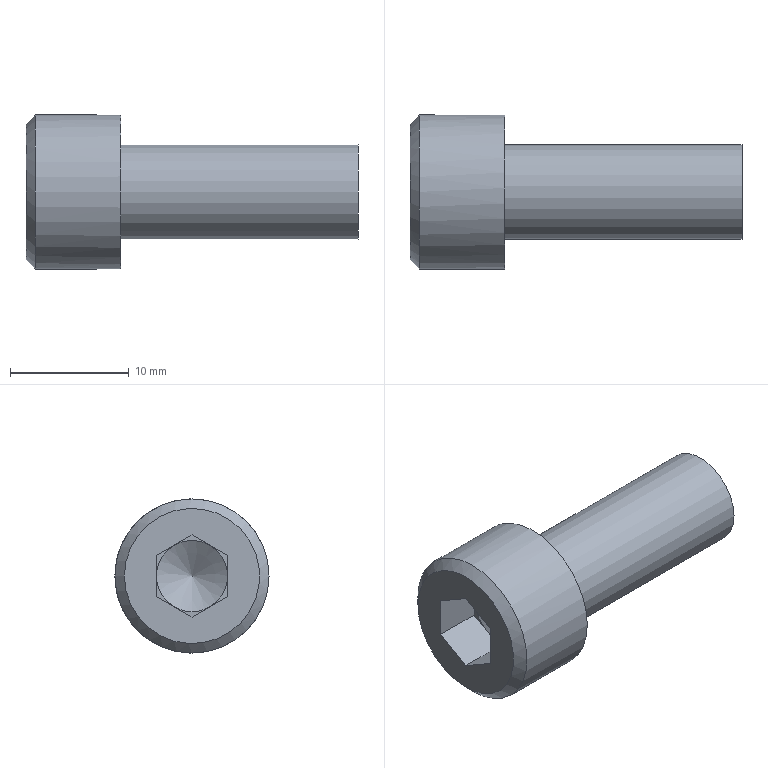Part | NX | features 5003_335_CB8-20 2 | 1 solid | 19 faces | box 28 x 13 x 13 mm | volume 1913 mm3 | plane 15 | cylinder 2 | cone 2 | commonest cylinder face diameters 8 x1 13 x1
STEP:
#1=CARTESIAN_POINT('',(-255.075,-520.3,-147.));
#2=VERTEX_POINT('',#1);
#3=CARTESIAN_POINT('',(-255.075,-526.,-147.));
#4=DIRECTION('',(1.,0.,0.));
#5=DIRECTION('',(0.,1.,0.));
#6=AXIS2_PLACEMENT_3D('',#3,#4,#5);
#7=CIRCLE('',#6,5.7);
#8=EDGE_CURVE('',#2,#2,#7,.F.);
#9=ORIENTED_EDGE('',*,*,#8,.T.);
#10=EDGE_LOOP('',(#9));
#11=FACE_BOUND('',#10,.T.);
#12=CARTESIAN_POINT('',(-255.075,-526.,-150.464));
#13=VERTEX_POINT('',#12);
#14=CARTESIAN_POINT('',(-255.075,-529.,-148.732));
#15=VERTEX_POINT('',#14);
#16=CARTESIAN_POINT('',(-255.075,-526.,-150.464));
#17=DIRECTION('',(0.,-0.866,0.5));
#18=VECTOR('',#17,1000.);
#19=LINE('',#16,#18);
#20=EDGE_CURVE('',#13,#15,#19,.T.);
#21=ORIENTED_EDGE('',*,*,#20,.F.);
#22=CARTESIAN_POINT('',(-255.075,-523.,-148.732));
#23=VERTEX_POINT('',#22);
#24=CARTESIAN_POINT('',(-255.075,-523.,-148.732));
#25=DIRECTION('',(0.,-0.866,-0.5));
#26=VECTOR('',#25,1000.);
#27=LINE('',#24,#26);
#28=EDGE_CURVE('',#23,#13,#27,.T.);
#29=ORIENTED_EDGE('',*,*,#28,.F.);
#30=CARTESIAN_POINT('',(-255.075,-523.,-145.268));
#31=VERTEX_POINT('',#30);
#32=CARTESIAN_POINT('',(-255.075,-523.,-145.268));
#33=DIRECTION('',(0.,0.,-1.));
#34=VECTOR('',#33,1000.);
#35=LINE('',#32,#34);
#36=EDGE_CURVE('',#31,#23,#35,.T.);
#37=ORIENTED_EDGE('',*,*,#36,.F.);
#38=CARTESIAN_POINT('',(-255.075,-526.,-143.536));
#39=VERTEX_POINT('',#38);
#40=CARTESIAN_POINT('',(-255.075,-526.,-143.536));
#41=DIRECTION('',(0.,0.866,-0.5));
#42=VECTOR('',#41,1000.);
#43=LINE('',#40,#42);
#44=EDGE_CURVE('',#39,#31,#43,.T.);
#45=ORIENTED_EDGE('',*,*,#44,.F.);
#46=CARTESIAN_POINT('',(-255.075,-529.,-145.268));
#47=VERTEX_POINT('',#46);
#48=CARTESIAN_POINT('',(-255.075,-529.,-145.268));
#49=DIRECTION('',(0.,0.866,0.5));
#50=VECTOR('',#49,1000.);
#51=LINE('',#48,#50);
#52=EDGE_CURVE('',#47,#39,#51,.T.);
#53=ORIENTED_EDGE('',*,*,#52,.F.);
#54=CARTESIAN_POINT('',(-255.075,-529.,-148.732));
#55=DIRECTION('',(0.,0.,1.));
#56=VECTOR('',#55,1000.);
#57=LINE('',#54,#56);
#58=EDGE_CURVE('',#15,#47,#57,.T.);
#59=ORIENTED_EDGE('',*,*,#58,.F.);
#60=EDGE_LOOP('',(#21,#29,#37,#45,#53,#59));
#61=FACE_BOUND('',#60,.T.);
#62=CARTESIAN_POINT('',(-255.075,-526.,-140.5));
#63=DIRECTION('',(1.,0.,0.));
#64=DIRECTION('',(0.,1.,0.));
#65=AXIS2_PLACEMENT_3D('',#62,#63,#64);
#66=PLANE('',#65);
#67=ADVANCED_FACE('',(#11,#61),#66,.F.);
#68=CARTESIAN_POINT('',(-227.075,-530.,-147.));
#69=VERTEX_POINT('',#68);
#70=CARTESIAN_POINT('',(-227.075,-526.,-147.));
#71=DIRECTION('',(-1.,0.,0.));
#72=DIRECTION('',(0.,-1.,0.));
#73=AXIS2_PLACEMENT_3D('',#70,#71,#72);
#74=CIRCLE('',#73,4.);
#75=EDGE_CURVE('',#69,#69,#74,.T.);
#76=ORIENTED_EDGE('',*,*,#75,.F.);
#77=EDGE_LOOP('',(#76));
#78=FACE_BOUND('',#77,.T.);
#79=CARTESIAN_POINT('',(-227.075,-526.,-147.));
#80=DIRECTION('',(-1.,0.,0.));
#81=DIRECTION('',(0.,-1.,0.));
#82=AXIS2_PLACEMENT_3D('',#79,#80,#81);
#83=PLANE('',#82);
#84=ADVANCED_FACE('',(#78),#83,.F.);
#85=CARTESIAN_POINT('',(-247.075,-530.,-147.));
#86=VERTEX_POINT('',#85);
#87=CARTESIAN_POINT('',(-247.075,-526.,-147.));
#88=DIRECTION('',(-1.,0.,0.));
#89=DIRECTION('',(0.,-1.,0.));
#90=AXIS2_PLACEMENT_3D('',#87,#88,#89);
#91=CIRCLE('',#90,4.);
#92=EDGE_CURVE('',#86,#86,#91,.T.);
#93=ORIENTED_EDGE('',*,*,#92,.F.);
#94=EDGE_LOOP('',(#93));
#95=FACE_BOUND('',#94,.T.);
#96=ORIENTED_EDGE('',*,*,#75,.T.);
#97=EDGE_LOOP('',(#96));
#98=FACE_BOUND('',#97,.T.);
#99=CARTESIAN_POINT('',(-255.075,-526.,-147.));
#100=DIRECTION('',(-1.,0.,0.));
#101=DIRECTION('',(0.,-1.,0.));
#102=AXIS2_PLACEMENT_3D('',#99,#100,#101);
#103=CYLINDRICAL_SURFACE('',#102,4.);
#104=ADVANCED_FACE('',(#95,#98),#103,.T.);
#105=CARTESIAN_POINT('',(-247.075,-532.5,-147.));
#106=VERTEX_POINT('',#105);
#107=CARTESIAN_POINT('',(-247.075,-526.,-147.));
#108=DIRECTION('',(-1.,0.,0.));
#109=DIRECTION('',(0.,-1.,0.));
#110=AXIS2_PLACEMENT_3D('',#107,#108,#109);
#111=CIRCLE('',#110,6.5);
#112=EDGE_CURVE('',#106,#106,#111,.T.);
#113=ORIENTED_EDGE('',*,*,#112,.F.);
#114=EDGE_LOOP('',(#113));
#115=FACE_BOUND('',#114,.T.);
#116=ORIENTED_EDGE('',*,*,#92,.T.);
#117=EDGE_LOOP('',(#116));
#118=FACE_BOUND('',#117,.T.);
#119=CARTESIAN_POINT('',(-247.075,-526.,-143.));
#120=DIRECTION('',(-1.,0.,0.));
#121=DIRECTION('',(0.,-1.,0.));
#122=AXIS2_PLACEMENT_3D('',#119,#120,#121);
#123=PLANE('',#122);
#124=ADVANCED_FACE('',(#115,#118),#123,.F.);
#125=CARTESIAN_POINT('',(-254.275,-519.5,-147.));
#126=VERTEX_POINT('',#125);
#127=CARTESIAN_POINT('',(-254.275,-526.,-147.));
#128=DIRECTION('',(1.,0.,0.));
#129=DIRECTION('',(0.,1.,0.));
#130=AXIS2_PLACEMENT_3D('',#127,#128,#129);
#131=CIRCLE('',#130,6.5);
#132=EDGE_CURVE('',#126,#126,#131,.T.);
#133=ORIENTED_EDGE('',*,*,#132,.T.);
#134=EDGE_LOOP('',(#133));
#135=FACE_BOUND('',#134,.T.);
#136=ORIENTED_EDGE('',*,*,#112,.T.);
#137=EDGE_LOOP('',(#136));
#138=FACE_BOUND('',#137,.T.);
#139=CARTESIAN_POINT('',(-255.075,-526.,-147.));
#140=DIRECTION('',(-1.,0.,0.));
#141=DIRECTION('',(0.,-1.,0.));
#142=AXIS2_PLACEMENT_3D('',#139,#140,#141);
#143=CYLINDRICAL_SURFACE('',#142,6.5);
#144=ADVANCED_FACE('',(#135,#138),#143,.T.);
#145=ORIENTED_EDGE('',*,*,#132,.F.);
#146=EDGE_LOOP('',(#145));
#147=FACE_BOUND('',#146,.T.);
#148=ORIENTED_EDGE('',*,*,#8,.F.);
#149=EDGE_LOOP('',(#148));
#150=FACE_BOUND('',#149,.T.);
#151=CARTESIAN_POINT('',(-255.075,-526.,-147.));
#152=DIRECTION('',(1.,0.,0.));
#153=DIRECTION('',(0.,1.,0.));
#154=AXIS2_PLACEMENT_3D('',#151,#152,#153);
#155=CONICAL_SURFACE('',#154,5.7,0.7854);
#156=ADVANCED_FACE('',(#147,#150),#155,.T.);
#157=CARTESIAN_POINT('',(-251.075,-523.,-148.732));
#158=VERTEX_POINT('',#157);
#159=CARTESIAN_POINT('',(-251.075,-524.5,-149.598));
#160=VERTEX_POINT('',#159);
#161=CARTESIAN_POINT('',(-251.075,-523.,-148.732));
#162=DIRECTION('',(0.,-0.866,-0.5));
#163=VECTOR('',#162,1000.);
#164=LINE('',#161,#163);
#165=EDGE_CURVE('',#158,#160,#164,.T.);
#166=ORIENTED_EDGE('',*,*,#165,.F.);
#167=CARTESIAN_POINT('',(-251.075,-523.,-148.732));
#168=DIRECTION('',(-1.,0.,0.));
#169=VECTOR('',#168,1000.);
#170=LINE('',#167,#169);
#171=EDGE_CURVE('',#158,#23,#170,.T.);
#172=ORIENTED_EDGE('',*,*,#171,.T.);
#173=ORIENTED_EDGE('',*,*,#28,.T.);
#174=CARTESIAN_POINT('',(-251.075,-526.,-150.464));
#175=VERTEX_POINT('',#174);
#176=CARTESIAN_POINT('',(-251.075,-526.,-150.464));
#177=DIRECTION('',(-1.,0.,0.));
#178=VECTOR('',#177,1000.);
#179=LINE('',#176,#178);
#180=EDGE_CURVE('',#175,#13,#179,.T.);
#181=ORIENTED_EDGE('',*,*,#180,.F.);
#182=CARTESIAN_POINT('',(-251.075,-523.,-148.732));
#183=DIRECTION('',(0.,-0.866,-0.5));
#184=VECTOR('',#183,1000.);
#185=LINE('',#182,#184);
#186=EDGE_CURVE('',#160,#175,#185,.T.);
#187=ORIENTED_EDGE('',*,*,#186,.F.);
#188=EDGE_LOOP('',(#166,#172,#173,#181,#187));
#189=FACE_BOUND('',#188,.T.);
#190=CARTESIAN_POINT('',(-251.075,-523.,-148.732));
#191=DIRECTION('',(0.,0.5,-0.866));
#192=DIRECTION('',(0.,0.866,0.5));
#193=AXIS2_PLACEMENT_3D('',#190,#191,#192);
#194=PLANE('',#193);
#195=ADVANCED_FACE('',(#189),#194,.F.);
#196=CARTESIAN_POINT('',(-251.075,-523.,-145.268));
#197=VERTEX_POINT('',#196);
#198=CARTESIAN_POINT('',(-251.075,-523.,-147.));
#199=VERTEX_POINT('',#198);
#200=CARTESIAN_POINT('',(-251.075,-523.,-145.268));
#201=DIRECTION('',(0.,0.,-1.));
#202=VECTOR('',#201,1000.);
#203=LINE('',#200,#202);
#204=EDGE_CURVE('',#197,#199,#203,.T.);
#205=ORIENTED_EDGE('',*,*,#204,.F.);
#206=CARTESIAN_POINT('',(-251.075,-523.,-145.268));
#207=DIRECTION('',(-1.,0.,0.));
#208=VECTOR('',#207,1000.);
#209=LINE('',#206,#208);
#210=EDGE_CURVE('',#197,#31,#209,.T.);
#211=ORIENTED_EDGE('',*,*,#210,.T.);
#212=ORIENTED_EDGE('',*,*,#36,.T.);
#213=ORIENTED_EDGE('',*,*,#171,.F.);
#214=CARTESIAN_POINT('',(-251.075,-523.,-145.268));
#215=DIRECTION('',(0.,0.,-1.));
#216=VECTOR('',#215,1000.);
#217=LINE('',#214,#216);
#218=EDGE_CURVE('',#199,#158,#217,.T.);
#219=ORIENTED_EDGE('',*,*,#218,.F.);
#220=EDGE_LOOP('',(#205,#211,#212,#213,#219));
#221=FACE_BOUND('',#220,.T.);
#222=CARTESIAN_POINT('',(-251.075,-523.,-145.268));
#223=DIRECTION('',(0.,1.,0.));
#224=DIRECTION('',(-1.,0.,0.));
#225=AXIS2_PLACEMENT_3D('',#222,#223,#224);
#226=PLANE('',#225);
#227=ADVANCED_FACE('',(#221),#226,.F.);
#228=CARTESIAN_POINT('',(-251.075,-526.,-143.536));
#229=VERTEX_POINT('',#228);
#230=CARTESIAN_POINT('',(-251.075,-524.5,-144.402));
#231=VERTEX_POINT('',#230);
#232=CARTESIAN_POINT('',(-251.075,-526.,-143.536));
#233=DIRECTION('',(0.,0.866,-0.5));
#234=VECTOR('',#233,1000.);
#235=LINE('',#232,#234);
#236=EDGE_CURVE('',#229,#231,#235,.T.);
#237=ORIENTED_EDGE('',*,*,#236,.F.);
#238=CARTESIAN_POINT('',(-251.075,-526.,-143.536));
#239=DIRECTION('',(-1.,0.,0.));
#240=VECTOR('',#239,1000.);
#241=LINE('',#238,#240);
#242=EDGE_CURVE('',#229,#39,#241,.T.);
#243=ORIENTED_EDGE('',*,*,#242,.T.);
#244=ORIENTED_EDGE('',*,*,#44,.T.);
#245=ORIENTED_EDGE('',*,*,#210,.F.);
#246=CARTESIAN_POINT('',(-251.075,-526.,-143.536));
#247=DIRECTION('',(0.,0.866,-0.5));
#248=VECTOR('',#247,1000.);
#249=LINE('',#246,#248);
#250=EDGE_CURVE('',#231,#197,#249,.T.);
#251=ORIENTED_EDGE('',*,*,#250,.F.);
#252=EDGE_LOOP('',(#237,#243,#244,#245,#251));
#253=FACE_BOUND('',#252,.T.);
#254=CARTESIAN_POINT('',(-251.075,-526.,-143.536));
#255=DIRECTION('',(0.,0.5,0.866));
#256=DIRECTION('',(0.,-0.866,0.5));
#257=AXIS2_PLACEMENT_3D('',#254,#255,#256);
#258=PLANE('',#257);
#259=ADVANCED_FACE('',(#253),#258,.F.);
#260=CARTESIAN_POINT('',(-251.075,-529.,-145.268));
#261=VERTEX_POINT('',#260);
#262=CARTESIAN_POINT('',(-251.075,-527.5,-144.402));
#263=VERTEX_POINT('',#262);
#264=CARTESIAN_POINT('',(-251.075,-529.,-145.268));
#265=DIRECTION('',(0.,0.866,0.5));
#266=VECTOR('',#265,1000.);
#267=LINE('',#264,#266);
#268=EDGE_CURVE('',#261,#263,#267,.T.);
#269=ORIENTED_EDGE('',*,*,#268,.F.);
#270=CARTESIAN_POINT('',(-251.075,-529.,-145.268));
#271=DIRECTION('',(-1.,0.,0.));
#272=VECTOR('',#271,1000.);
#273=LINE('',#270,#272);
#274=EDGE_CURVE('',#261,#47,#273,.T.);
#275=ORIENTED_EDGE('',*,*,#274,.T.);
#276=ORIENTED_EDGE('',*,*,#52,.T.);
#277=ORIENTED_EDGE('',*,*,#242,.F.);
#278=CARTESIAN_POINT('',(-251.075,-529.,-145.268));
#279=DIRECTION('',(0.,0.866,0.5));
#280=VECTOR('',#279,1000.);
#281=LINE('',#278,#280);
#282=EDGE_CURVE('',#263,#229,#281,.T.);
#283=ORIENTED_EDGE('',*,*,#282,.F.);
#284=EDGE_LOOP('',(#269,#275,#276,#277,#283));
#285=FACE_BOUND('',#284,.T.);
#286=CARTESIAN_POINT('',(-251.075,-529.,-145.268));
#287=DIRECTION('',(0.,-0.5,0.866));
#288=DIRECTION('',(0.,-0.866,-0.5));
#289=AXIS2_PLACEMENT_3D('',#286,#287,#288);
#290=PLANE('',#289);
#291=ADVANCED_FACE('',(#285),#290,.F.);
#292=CARTESIAN_POINT('',(-251.075,-529.,-148.732));
#293=VERTEX_POINT('',#292);
#294=CARTESIAN_POINT('',(-251.075,-529.,-147.));
#295=VERTEX_POINT('',#294);
#296=CARTESIAN_POINT('',(-251.075,-529.,-148.732));
#297=DIRECTION('',(0.,0.,1.));
#298=VECTOR('',#297,1000.);
#299=LINE('',#296,#298);
#300=EDGE_CURVE('',#293,#295,#299,.T.);
#301=ORIENTED_EDGE('',*,*,#300,.F.);
#302=CARTESIAN_POINT('',(-251.075,-529.,-148.732));
#303=DIRECTION('',(-1.,0.,0.));
#304=VECTOR('',#303,1000.);
#305=LINE('',#302,#304);
#306=EDGE_CURVE('',#293,#15,#305,.T.);
#307=ORIENTED_EDGE('',*,*,#306,.T.);
#308=ORIENTED_EDGE('',*,*,#58,.T.);
#309=ORIENTED_EDGE('',*,*,#274,.F.);
#310=CARTESIAN_POINT('',(-251.075,-529.,-148.732));
#311=DIRECTION('',(0.,0.,1.));
#312=VECTOR('',#311,1000.);
#313=LINE('',#310,#312);
#314=EDGE_CURVE('',#295,#261,#313,.T.);
#315=ORIENTED_EDGE('',*,*,#314,.F.);
#316=EDGE_LOOP('',(#301,#307,#308,#309,#315));
#317=FACE_BOUND('',#316,.T.);
#318=CARTESIAN_POINT('',(-251.075,-529.,-148.732));
#319=DIRECTION('',(0.,-1.,0.));
#320=DIRECTION('',(0.,0.,-1.));
#321=AXIS2_PLACEMENT_3D('',#318,#319,#320);
#322=PLANE('',#321);
#323=ADVANCED_FACE('',(#317),#322,.F.);
#324=CARTESIAN_POINT('',(-251.075,-527.5,-149.598));
#325=VERTEX_POINT('',#324);
#326=CARTESIAN_POINT('',(-251.075,-526.,-150.464));
#327=DIRECTION('',(0.,-0.866,0.5));
#328=VECTOR('',#327,1000.);
#329=LINE('',#326,#328);
#330=EDGE_CURVE('',#175,#325,#329,.T.);
#331=ORIENTED_EDGE('',*,*,#330,.F.);
#332=ORIENTED_EDGE('',*,*,#180,.T.);
#333=ORIENTED_EDGE('',*,*,#20,.T.);
#334=ORIENTED_EDGE('',*,*,#306,.F.);
#335=CARTESIAN_POINT('',(-251.075,-526.,-150.464));
#336=DIRECTION('',(0.,-0.866,0.5));
#337=VECTOR('',#336,1000.);
#338=LINE('',#335,#337);
#339=EDGE_CURVE('',#325,#293,#338,.T.);
#340=ORIENTED_EDGE('',*,*,#339,.F.);
#341=EDGE_LOOP('',(#331,#332,#333,#334,#340));
#342=FACE_BOUND('',#341,.T.);
#343=CARTESIAN_POINT('',(-251.075,-526.,-150.464));
#344=DIRECTION('',(0.,-0.5,-0.866));
#345=DIRECTION('',(0.,0.866,-0.5));
#346=AXIS2_PLACEMENT_3D('',#343,#344,#345);
#347=PLANE('',#346);
#348=ADVANCED_FACE('',(#342),#347,.F.);
#349=ORIENTED_EDGE('',*,*,#314,.T.);
#350=ORIENTED_EDGE('',*,*,#268,.T.);
#351=CARTESIAN_POINT('',(-251.075,-526.,-147.));
#352=DIRECTION('',(-1.,0.,0.));
#353=DIRECTION('',(0.,0.,-1.));
#354=AXIS2_PLACEMENT_3D('',#351,#352,#353);
#355=CIRCLE('',#354,3.);
#356=EDGE_CURVE('',#295,#263,#355,.T.);
#357=ORIENTED_EDGE('',*,*,#356,.F.);
#358=EDGE_LOOP('',(#349,#350,#357));
#359=FACE_BOUND('',#358,.T.);
#360=CARTESIAN_POINT('',(-251.075,-526.,-147.));
#361=DIRECTION('',(-1.,0.,0.));
#362=DIRECTION('',(0.,-1.,0.));
#363=AXIS2_PLACEMENT_3D('',#360,#361,#362);
#364=PLANE('',#363);
#365=ADVANCED_FACE('',(#359),#364,.T.);
#366=ORIENTED_EDGE('',*,*,#282,.T.);
#367=ORIENTED_EDGE('',*,*,#236,.T.);
#368=CARTESIAN_POINT('',(-251.075,-526.,-147.));
#369=DIRECTION('',(-1.,0.,0.));
#370=DIRECTION('',(0.,0.,-1.));
#371=AXIS2_PLACEMENT_3D('',#368,#369,#370);
#372=CIRCLE('',#371,3.);
#373=EDGE_CURVE('',#263,#231,#372,.T.);
#374=ORIENTED_EDGE('',*,*,#373,.F.);
#375=EDGE_LOOP('',(#366,#367,#374));
#376=FACE_BOUND('',#375,.T.);
#377=CARTESIAN_POINT('',(-251.075,-526.,-147.));
#378=DIRECTION('',(-1.,0.,0.));
#379=DIRECTION('',(0.,-1.,0.));
#380=AXIS2_PLACEMENT_3D('',#377,#378,#379);
#381=PLANE('',#380);
#382=ADVANCED_FACE('',(#376),#381,.T.);
#383=ORIENTED_EDGE('',*,*,#250,.T.);
#384=ORIENTED_EDGE('',*,*,#204,.T.);
#385=CARTESIAN_POINT('',(-251.075,-526.,-147.));
#386=DIRECTION('',(-1.,0.,0.));
#387=DIRECTION('',(0.,0.,-1.));
#388=AXIS2_PLACEMENT_3D('',#385,#386,#387);
#389=CIRCLE('',#388,3.);
#390=EDGE_CURVE('',#231,#199,#389,.T.);
#391=ORIENTED_EDGE('',*,*,#390,.F.);
#392=EDGE_LOOP('',(#383,#384,#391));
#393=FACE_BOUND('',#392,.T.);
#394=CARTESIAN_POINT('',(-251.075,-526.,-147.));
#395=DIRECTION('',(-1.,0.,0.));
#396=DIRECTION('',(0.,-1.,0.));
#397=AXIS2_PLACEMENT_3D('',#394,#395,#396);
#398=PLANE('',#397);
#399=ADVANCED_FACE('',(#393),#398,.T.);
#400=ORIENTED_EDGE('',*,*,#218,.T.);
#401=ORIENTED_EDGE('',*,*,#165,.T.);
#402=CARTESIAN_POINT('',(-251.075,-526.,-147.));
#403=DIRECTION('',(-1.,0.,0.));
#404=DIRECTION('',(0.,0.,-1.));
#405=AXIS2_PLACEMENT_3D('',#402,#403,#404);
#406=CIRCLE('',#405,3.);
#407=EDGE_CURVE('',#199,#160,#406,.T.);
#408=ORIENTED_EDGE('',*,*,#407,.F.);
#409=EDGE_LOOP('',(#400,#401,#408));
#410=FACE_BOUND('',#409,.T.);
#411=CARTESIAN_POINT('',(-251.075,-526.,-147.));
#412=DIRECTION('',(-1.,0.,0.));
#413=DIRECTION('',(0.,-1.,0.));
#414=AXIS2_PLACEMENT_3D('',#411,#412,#413);
#415=PLANE('',#414);
#416=ADVANCED_FACE('',(#410),#415,.T.);
#417=ORIENTED_EDGE('',*,*,#186,.T.);
#418=ORIENTED_EDGE('',*,*,#330,.T.);
#419=CARTESIAN_POINT('',(-251.075,-526.,-147.));
#420=DIRECTION('',(-1.,0.,0.));
#421=DIRECTION('',(0.,0.,-1.));
#422=AXIS2_PLACEMENT_3D('',#419,#420,#421);
#423=CIRCLE('',#422,3.);
#424=EDGE_CURVE('',#160,#325,#423,.T.);
#425=ORIENTED_EDGE('',*,*,#424,.F.);
#426=EDGE_LOOP('',(#417,#418,#425));
#427=FACE_BOUND('',#426,.T.);
#428=CARTESIAN_POINT('',(-251.075,-526.,-147.));
#429=DIRECTION('',(-1.,0.,0.));
#430=DIRECTION('',(0.,-1.,0.));
#431=AXIS2_PLACEMENT_3D('',#428,#429,#430);
#432=PLANE('',#431);
#433=ADVANCED_FACE('',(#427),#432,.T.);
#434=ORIENTED_EDGE('',*,*,#339,.T.);
#435=ORIENTED_EDGE('',*,*,#300,.T.);
#436=CARTESIAN_POINT('',(-251.075,-526.,-147.));
#437=DIRECTION('',(-1.,0.,0.));
#438=DIRECTION('',(0.,0.,-1.));
#439=AXIS2_PLACEMENT_3D('',#436,#437,#438);
#440=CIRCLE('',#439,3.);
#441=EDGE_CURVE('',#325,#295,#440,.T.);
#442=ORIENTED_EDGE('',*,*,#441,.F.);
#443=EDGE_LOOP('',(#434,#435,#442));
#444=FACE_BOUND('',#443,.T.);
#445=CARTESIAN_POINT('',(-251.075,-526.,-147.));
#446=DIRECTION('',(-1.,0.,0.));
#447=DIRECTION('',(0.,-1.,0.));
#448=AXIS2_PLACEMENT_3D('',#445,#446,#447);
#449=PLANE('',#448);
#450=ADVANCED_FACE('',(#444),#449,.T.);
#451=ORIENTED_EDGE('',*,*,#441,.T.);
#452=ORIENTED_EDGE('',*,*,#356,.T.);
#453=ORIENTED_EDGE('',*,*,#373,.T.);
#454=ORIENTED_EDGE('',*,*,#390,.T.);
#455=ORIENTED_EDGE('',*,*,#407,.T.);
#456=ORIENTED_EDGE('',*,*,#424,.T.);
#457=EDGE_LOOP('',(#451,#452,#453,#454,#455,#456));
#458=FACE_BOUND('',#457,.T.);
#459=CARTESIAN_POINT('',(-249.272,-526.,-147.));
#460=VERTEX_POINT('',#459);
#461=VERTEX_LOOP('',#460);
#462=FACE_BOUND('',#461,.T.);
#463=CARTESIAN_POINT('',(-249.272,-526.,-147.));
#464=DIRECTION('',(-1.,0.,0.));
#465=DIRECTION('',(0.,0.,-1.));
#466=AXIS2_PLACEMENT_3D('',#463,#464,#465);
#467=CONICAL_SURFACE('',#466,0.,1.03);
#468=ADVANCED_FACE('',(#458,#462),#467,.F.);
#469=CLOSED_SHELL('',(#67,#84,#104,#124,#144,#156,#195,#227,#259,#291,#323,#348,#365,#382,#399,#416,#433,#450,#468));
#470=MANIFOLD_SOLID_BREP('',#469);
#471=(LENGTH_UNIT()NAMED_UNIT(*)SI_UNIT(.MILLI.,.METRE.));
#472=UNCERTAINTY_MEASURE_WITH_UNIT(LENGTH_MEASURE(0.00001),#471,'','');
#473=(NAMED_UNIT(*)PLANE_ANGLE_UNIT()SI_UNIT($,.RADIAN.));
#474=(NAMED_UNIT(*)SI_UNIT($,.STERADIAN.)SOLID_ANGLE_UNIT());
#475=(GEOMETRIC_REPRESENTATION_CONTEXT(3)GLOBAL_UNCERTAINTY_ASSIGNED_CONTEXT((#472))GLOBAL_UNIT_ASSIGNED_CONTEXT((#471,#473,#474))REPRESENTATION_CONTEXT('',''));
#476=ADVANCED_BREP_SHAPE_REPRESENTATION('',(#470),#475);